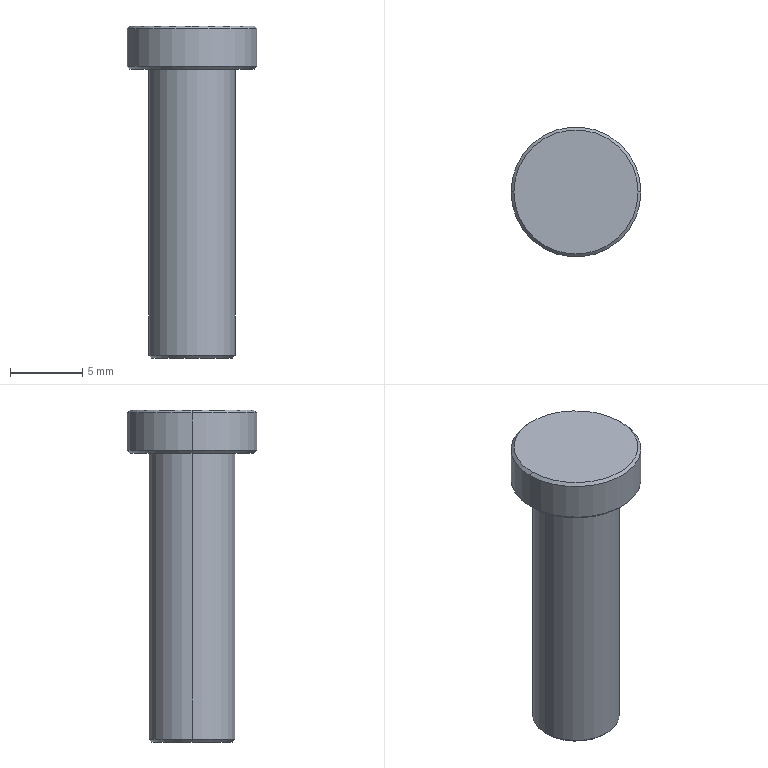Part | SolidWorks | features Chamfer 1, Extrusion 1, ICE 1 | 1 solid | 13 faces | box 9 x 9 x 23 mm | volume 754.856 mm3 | cone 6 | cylinder 4 | plane 3 | commonest cylinder face diameters 6 x2 9 x2
STEP:
#1=CARTESIAN_POINT('',(-2.8,0.,0.));
#2=VERTEX_POINT('',#1);
#3=CARTESIAN_POINT('',(2.8,0.,0.));
#4=VERTEX_POINT('',#3);
#5=CARTESIAN_POINT('',(0.,0.,0.));
#6=DIRECTION('',(0.,0.,-1.));
#7=DIRECTION('',(1.,0.,0.));
#8=AXIS2_PLACEMENT_3D('',#5,#6,#7);
#9=CIRCLE('',#8,2.8);
#10=EDGE_CURVE('',#2,#4,#9,.T.);
#11=ORIENTED_EDGE('',*,*,#10,.F.);
#12=CARTESIAN_POINT('',(-3.,0.,0.2));
#13=VERTEX_POINT('',#12);
#14=CARTESIAN_POINT('',(-3.,0.,0.2));
#15=DIRECTION('',(-0.7071,0.,0.7071));
#16=VECTOR('',#15,1000.);
#17=LINE('',#14,#16);
#18=EDGE_CURVE('',#2,#13,#17,.T.);
#19=ORIENTED_EDGE('',*,*,#18,.T.);
#20=CARTESIAN_POINT('',(3.,0.,0.2));
#21=VERTEX_POINT('',#20);
#22=CARTESIAN_POINT('',(0.,0.,0.2));
#23=DIRECTION('',(0.,0.,1.));
#24=DIRECTION('',(1.,0.,0.));
#25=AXIS2_PLACEMENT_3D('',#22,#23,#24);
#26=CIRCLE('',#25,3.);
#27=EDGE_CURVE('',#21,#13,#26,.T.);
#28=ORIENTED_EDGE('',*,*,#27,.F.);
#29=CARTESIAN_POINT('',(3.,0.,0.2));
#30=DIRECTION('',(0.7071,0.,0.7071));
#31=VECTOR('',#30,1000.);
#32=LINE('',#29,#31);
#33=EDGE_CURVE('',#4,#21,#32,.T.);
#34=ORIENTED_EDGE('',*,*,#33,.F.);
#35=EDGE_LOOP('',(#11,#19,#28,#34));
#36=FACE_OUTER_BOUND('',#35,.T.);
#37=CARTESIAN_POINT('',(0.,0.,0.2));
#38=DIRECTION('',(0.,0.,1.));
#39=DIRECTION('',(1.,0.,0.));
#40=AXIS2_PLACEMENT_3D('',#37,#38,#39);
#41=CONICAL_SURFACE('',#40,3.,0.7854);
#42=ADVANCED_FACE('',(#36),#41,.T.);
#43=CARTESIAN_POINT('',(-4.3,0.,20.));
#44=VERTEX_POINT('',#43);
#45=CARTESIAN_POINT('',(4.3,0.,20.));
#46=VERTEX_POINT('',#45);
#47=CARTESIAN_POINT('',(0.,0.,20.));
#48=DIRECTION('',(0.,0.,-1.));
#49=DIRECTION('',(1.,0.,0.));
#50=AXIS2_PLACEMENT_3D('',#47,#48,#49);
#51=CIRCLE('',#50,4.3);
#52=EDGE_CURVE('',#44,#46,#51,.T.);
#53=ORIENTED_EDGE('',*,*,#52,.F.);
#54=CARTESIAN_POINT('',(-4.5,0.,20.2));
#55=VERTEX_POINT('',#54);
#56=CARTESIAN_POINT('',(-4.5,0.,20.2));
#57=DIRECTION('',(-0.7071,0.,0.7071));
#58=VECTOR('',#57,1000.);
#59=LINE('',#56,#58);
#60=EDGE_CURVE('',#44,#55,#59,.T.);
#61=ORIENTED_EDGE('',*,*,#60,.T.);
#62=CARTESIAN_POINT('',(4.5,0.,20.2));
#63=VERTEX_POINT('',#62);
#64=CARTESIAN_POINT('',(0.,0.,20.2));
#65=DIRECTION('',(0.,0.,1.));
#66=DIRECTION('',(1.,0.,0.));
#67=AXIS2_PLACEMENT_3D('',#64,#65,#66);
#68=CIRCLE('',#67,4.5);
#69=EDGE_CURVE('',#63,#55,#68,.T.);
#70=ORIENTED_EDGE('',*,*,#69,.F.);
#71=CARTESIAN_POINT('',(4.5,0.,20.2));
#72=DIRECTION('',(0.7071,0.,0.7071));
#73=VECTOR('',#72,1000.);
#74=LINE('',#71,#73);
#75=EDGE_CURVE('',#46,#63,#74,.T.);
#76=ORIENTED_EDGE('',*,*,#75,.F.);
#77=EDGE_LOOP('',(#53,#61,#70,#76));
#78=FACE_OUTER_BOUND('',#77,.T.);
#79=CARTESIAN_POINT('',(0.,0.,20.2));
#80=DIRECTION('',(0.,0.,1.));
#81=DIRECTION('',(1.,0.,0.));
#82=AXIS2_PLACEMENT_3D('',#79,#80,#81);
#83=CONICAL_SURFACE('',#82,4.5,0.7854);
#84=ADVANCED_FACE('',(#78),#83,.T.);
#85=CARTESIAN_POINT('',(4.3,0.,23.));
#86=VERTEX_POINT('',#85);
#87=CARTESIAN_POINT('',(-4.3,0.,23.));
#88=VERTEX_POINT('',#87);
#89=CARTESIAN_POINT('',(0.,0.,23.));
#90=DIRECTION('',(0.,0.,1.));
#91=DIRECTION('',(1.,0.,0.));
#92=AXIS2_PLACEMENT_3D('',#89,#90,#91);
#93=CIRCLE('',#92,4.3);
#94=EDGE_CURVE('',#86,#88,#93,.T.);
#95=ORIENTED_EDGE('',*,*,#94,.F.);
#96=CARTESIAN_POINT('',(4.5,0.,22.8));
#97=VERTEX_POINT('',#96);
#98=CARTESIAN_POINT('',(4.3,0.,23.));
#99=DIRECTION('',(0.7071,0.,-0.7071));
#100=VECTOR('',#99,1000.);
#101=LINE('',#98,#100);
#102=EDGE_CURVE('',#86,#97,#101,.T.);
#103=ORIENTED_EDGE('',*,*,#102,.T.);
#104=CARTESIAN_POINT('',(-4.5,0.,22.8));
#105=VERTEX_POINT('',#104);
#106=CARTESIAN_POINT('',(0.,0.,22.8));
#107=DIRECTION('',(0.,0.,-1.));
#108=DIRECTION('',(1.,0.,0.));
#109=AXIS2_PLACEMENT_3D('',#106,#107,#108);
#110=CIRCLE('',#109,4.5);
#111=EDGE_CURVE('',#105,#97,#110,.T.);
#112=ORIENTED_EDGE('',*,*,#111,.F.);
#113=CARTESIAN_POINT('',(-4.3,0.,23.));
#114=DIRECTION('',(-0.7071,0.,-0.7071));
#115=VECTOR('',#114,1000.);
#116=LINE('',#113,#115);
#117=EDGE_CURVE('',#88,#105,#116,.T.);
#118=ORIENTED_EDGE('',*,*,#117,.F.);
#119=EDGE_LOOP('',(#95,#103,#112,#118));
#120=FACE_OUTER_BOUND('',#119,.T.);
#121=CARTESIAN_POINT('',(0.,0.,23.));
#122=DIRECTION('',(0.,0.,-1.));
#123=DIRECTION('',(-1.,0.,0.));
#124=AXIS2_PLACEMENT_3D('',#121,#122,#123);
#125=CONICAL_SURFACE('',#124,4.3,0.7854);
#126=ADVANCED_FACE('',(#120),#125,.T.);
#127=ORIENTED_EDGE('',*,*,#111,.T.);
#128=CARTESIAN_POINT('',(4.5,0.,23.));
#129=DIRECTION('',(0.,0.,-1.));
#130=VECTOR('',#129,1000.);
#131=LINE('',#128,#130);
#132=EDGE_CURVE('',#97,#63,#131,.T.);
#133=ORIENTED_EDGE('',*,*,#132,.T.);
#134=ORIENTED_EDGE('',*,*,#69,.T.);
#135=CARTESIAN_POINT('',(-4.5,0.,23.));
#136=DIRECTION('',(0.,0.,-1.));
#137=VECTOR('',#136,1000.);
#138=LINE('',#135,#137);
#139=EDGE_CURVE('',#105,#55,#138,.T.);
#140=ORIENTED_EDGE('',*,*,#139,.F.);
#141=EDGE_LOOP('',(#127,#133,#134,#140));
#142=FACE_OUTER_BOUND('',#141,.T.);
#143=CARTESIAN_POINT('',(0.,0.,23.));
#144=DIRECTION('',(0.,0.,-1.));
#145=DIRECTION('',(-1.,0.,0.));
#146=AXIS2_PLACEMENT_3D('',#143,#144,#145);
#147=CYLINDRICAL_SURFACE('',#146,4.5);
#148=ADVANCED_FACE('',(#142),#147,.T.);
#149=CARTESIAN_POINT('',(3.,0.,20.));
#150=VERTEX_POINT('',#149);
#151=CARTESIAN_POINT('',(-3.,0.,20.));
#152=VERTEX_POINT('',#151);
#153=CARTESIAN_POINT('',(0.,0.,20.));
#154=DIRECTION('',(0.,0.,1.));
#155=DIRECTION('',(1.,0.,0.));
#156=AXIS2_PLACEMENT_3D('',#153,#154,#155);
#157=CIRCLE('',#156,3.);
#158=EDGE_CURVE('',#150,#152,#157,.T.);
#159=ORIENTED_EDGE('',*,*,#158,.F.);
#160=CARTESIAN_POINT('',(3.,0.,20.));
#161=DIRECTION('',(0.,0.,-1.));
#162=VECTOR('',#161,1000.);
#163=LINE('',#160,#162);
#164=EDGE_CURVE('',#150,#21,#163,.T.);
#165=ORIENTED_EDGE('',*,*,#164,.T.);
#166=ORIENTED_EDGE('',*,*,#27,.T.);
#167=CARTESIAN_POINT('',(-3.,0.,20.));
#168=DIRECTION('',(0.,0.,-1.));
#169=VECTOR('',#168,1000.);
#170=LINE('',#167,#169);
#171=EDGE_CURVE('',#152,#13,#170,.T.);
#172=ORIENTED_EDGE('',*,*,#171,.F.);
#173=EDGE_LOOP('',(#159,#165,#166,#172));
#174=FACE_OUTER_BOUND('',#173,.T.);
#175=CARTESIAN_POINT('',(0.,0.,20.));
#176=DIRECTION('',(0.,0.,-1.));
#177=DIRECTION('',(-1.,0.,0.));
#178=AXIS2_PLACEMENT_3D('',#175,#176,#177);
#179=CYLINDRICAL_SURFACE('',#178,3.);
#180=ADVANCED_FACE('',(#174),#179,.T.);
#181=ORIENTED_EDGE('',*,*,#164,.F.);
#182=CARTESIAN_POINT('',(0.,0.,20.));
#183=DIRECTION('',(0.,0.,1.));
#184=DIRECTION('',(1.,0.,0.));
#185=AXIS2_PLACEMENT_3D('',#182,#183,#184);
#186=CIRCLE('',#185,3.);
#187=EDGE_CURVE('',#152,#150,#186,.T.);
#188=ORIENTED_EDGE('',*,*,#187,.F.);
#189=ORIENTED_EDGE('',*,*,#171,.T.);
#190=CARTESIAN_POINT('',(0.,0.,0.2));
#191=DIRECTION('',(0.,0.,1.));
#192=DIRECTION('',(1.,0.,0.));
#193=AXIS2_PLACEMENT_3D('',#190,#191,#192);
#194=CIRCLE('',#193,3.);
#195=EDGE_CURVE('',#13,#21,#194,.T.);
#196=ORIENTED_EDGE('',*,*,#195,.T.);
#197=EDGE_LOOP('',(#181,#188,#189,#196));
#198=FACE_OUTER_BOUND('',#197,.T.);
#199=CARTESIAN_POINT('',(0.,0.,20.));
#200=DIRECTION('',(0.,0.,-1.));
#201=DIRECTION('',(-1.,0.,0.));
#202=AXIS2_PLACEMENT_3D('',#199,#200,#201);
#203=CYLINDRICAL_SURFACE('',#202,3.);
#204=ADVANCED_FACE('',(#198),#203,.T.);
#205=CARTESIAN_POINT('',(0.,0.,0.));
#206=DIRECTION('',(0.,0.,-1.));
#207=DIRECTION('',(1.,0.,0.));
#208=AXIS2_PLACEMENT_3D('',#205,#206,#207);
#209=CIRCLE('',#208,2.8);
#210=EDGE_CURVE('',#4,#2,#209,.T.);
#211=ORIENTED_EDGE('',*,*,#210,.T.);
#212=ORIENTED_EDGE('',*,*,#10,.T.);
#213=EDGE_LOOP('',(#211,#212));
#214=FACE_OUTER_BOUND('',#213,.T.);
#215=CARTESIAN_POINT('',(0.,0.,0.));
#216=DIRECTION('',(0.,0.,1.));
#217=DIRECTION('',(1.,0.,0.));
#218=AXIS2_PLACEMENT_3D('',#215,#216,#217);
#219=PLANE('',#218);
#220=ADVANCED_FACE('',(#214),#219,.F.);
#221=ORIENTED_EDGE('',*,*,#132,.F.);
#222=CARTESIAN_POINT('',(0.,0.,22.8));
#223=DIRECTION('',(0.,0.,-1.));
#224=DIRECTION('',(1.,0.,0.));
#225=AXIS2_PLACEMENT_3D('',#222,#223,#224);
#226=CIRCLE('',#225,4.5);
#227=EDGE_CURVE('',#97,#105,#226,.T.);
#228=ORIENTED_EDGE('',*,*,#227,.T.);
#229=ORIENTED_EDGE('',*,*,#139,.T.);
#230=CARTESIAN_POINT('',(0.,0.,20.2));
#231=DIRECTION('',(0.,0.,1.));
#232=DIRECTION('',(1.,0.,0.));
#233=AXIS2_PLACEMENT_3D('',#230,#231,#232);
#234=CIRCLE('',#233,4.5);
#235=EDGE_CURVE('',#55,#63,#234,.T.);
#236=ORIENTED_EDGE('',*,*,#235,.T.);
#237=EDGE_LOOP('',(#221,#228,#229,#236));
#238=FACE_OUTER_BOUND('',#237,.T.);
#239=CARTESIAN_POINT('',(0.,0.,23.));
#240=DIRECTION('',(0.,0.,-1.));
#241=DIRECTION('',(-1.,0.,0.));
#242=AXIS2_PLACEMENT_3D('',#239,#240,#241);
#243=CYLINDRICAL_SURFACE('',#242,4.5);
#244=ADVANCED_FACE('',(#238),#243,.T.);
#245=CARTESIAN_POINT('',(0.,0.,23.));
#246=DIRECTION('',(0.,0.,1.));
#247=DIRECTION('',(1.,0.,0.));
#248=AXIS2_PLACEMENT_3D('',#245,#246,#247);
#249=CIRCLE('',#248,4.3);
#250=EDGE_CURVE('',#88,#86,#249,.T.);
#251=ORIENTED_EDGE('',*,*,#250,.T.);
#252=ORIENTED_EDGE('',*,*,#94,.T.);
#253=EDGE_LOOP('',(#251,#252));
#254=FACE_OUTER_BOUND('',#253,.T.);
#255=CARTESIAN_POINT('',(0.,0.,23.));
#256=DIRECTION('',(0.,0.,1.));
#257=DIRECTION('',(1.,0.,0.));
#258=AXIS2_PLACEMENT_3D('',#255,#256,#257);
#259=PLANE('',#258);
#260=ADVANCED_FACE('',(#254),#259,.T.);
#261=CARTESIAN_POINT('',(0.,0.,20.));
#262=DIRECTION('',(0.,0.,-1.));
#263=DIRECTION('',(1.,0.,0.));
#264=AXIS2_PLACEMENT_3D('',#261,#262,#263);
#265=CIRCLE('',#264,4.3);
#266=EDGE_CURVE('',#46,#44,#265,.T.);
#267=ORIENTED_EDGE('',*,*,#266,.T.);
#268=ORIENTED_EDGE('',*,*,#52,.T.);
#269=EDGE_LOOP('',(#267,#268));
#270=FACE_OUTER_BOUND('',#269,.T.);
#271=ORIENTED_EDGE('',*,*,#187,.T.);
#272=ORIENTED_EDGE('',*,*,#158,.T.);
#273=EDGE_LOOP('',(#271,#272));
#274=FACE_BOUND('',#273,.T.);
#275=CARTESIAN_POINT('',(0.,0.,20.));
#276=DIRECTION('',(0.,0.,1.));
#277=DIRECTION('',(1.,0.,0.));
#278=AXIS2_PLACEMENT_3D('',#275,#276,#277);
#279=PLANE('',#278);
#280=ADVANCED_FACE('',(#270,#274),#279,.F.);
#281=ORIENTED_EDGE('',*,*,#102,.F.);
#282=ORIENTED_EDGE('',*,*,#250,.F.);
#283=ORIENTED_EDGE('',*,*,#117,.T.);
#284=ORIENTED_EDGE('',*,*,#227,.F.);
#285=EDGE_LOOP('',(#281,#282,#283,#284));
#286=FACE_OUTER_BOUND('',#285,.T.);
#287=CARTESIAN_POINT('',(0.,0.,23.));
#288=DIRECTION('',(0.,0.,-1.));
#289=DIRECTION('',(-1.,0.,0.));
#290=AXIS2_PLACEMENT_3D('',#287,#288,#289);
#291=CONICAL_SURFACE('',#290,4.3,0.7854);
#292=ADVANCED_FACE('',(#286),#291,.T.);
#293=ORIENTED_EDGE('',*,*,#60,.F.);
#294=ORIENTED_EDGE('',*,*,#266,.F.);
#295=ORIENTED_EDGE('',*,*,#75,.T.);
#296=ORIENTED_EDGE('',*,*,#235,.F.);
#297=EDGE_LOOP('',(#293,#294,#295,#296));
#298=FACE_OUTER_BOUND('',#297,.T.);
#299=CARTESIAN_POINT('',(0.,0.,20.2));
#300=DIRECTION('',(0.,0.,1.));
#301=DIRECTION('',(1.,0.,0.));
#302=AXIS2_PLACEMENT_3D('',#299,#300,#301);
#303=CONICAL_SURFACE('',#302,4.5,0.7854);
#304=ADVANCED_FACE('',(#298),#303,.T.);
#305=ORIENTED_EDGE('',*,*,#18,.F.);
#306=ORIENTED_EDGE('',*,*,#210,.F.);
#307=ORIENTED_EDGE('',*,*,#33,.T.);
#308=ORIENTED_EDGE('',*,*,#195,.F.);
#309=EDGE_LOOP('',(#305,#306,#307,#308));
#310=FACE_OUTER_BOUND('',#309,.T.);
#311=CARTESIAN_POINT('',(0.,0.,0.2));
#312=DIRECTION('',(0.,0.,1.));
#313=DIRECTION('',(1.,0.,0.));
#314=AXIS2_PLACEMENT_3D('',#311,#312,#313);
#315=CONICAL_SURFACE('',#314,3.,0.7854);
#316=ADVANCED_FACE('',(#310),#315,.T.);
#317=CLOSED_SHELL('',(#42,#84,#126,#148,#180,#204,#220,#244,#260,#280,#292,#304,#316));
#318=MANIFOLD_SOLID_BREP('',#317);
#319=CARTESIAN_POINT('',(0.,0.,0.));
#320=DIRECTION('',(0.,0.,1.));
#321=DIRECTION('',(1.,0.,0.));
#322=AXIS2_PLACEMENT_3D('',#319,#320,#321);
#323=(LENGTH_UNIT()NAMED_UNIT(*)SI_UNIT(.MILLI.,.METRE.));
#324=UNCERTAINTY_MEASURE_WITH_UNIT(LENGTH_MEASURE(0.00001),#323,'','');
#325=(NAMED_UNIT(*)PLANE_ANGLE_UNIT()SI_UNIT($,.RADIAN.));
#326=(NAMED_UNIT(*)SI_UNIT($,.STERADIAN.)SOLID_ANGLE_UNIT());
#327=(GEOMETRIC_REPRESENTATION_CONTEXT(3)GLOBAL_UNCERTAINTY_ASSIGNED_CONTEXT((#324))GLOBAL_UNIT_ASSIGNED_CONTEXT((#323,#325,#326))REPRESENTATION_CONTEXT('',''));
#328=ADVANCED_BREP_SHAPE_REPRESENTATION('',(#318,#322),#327);